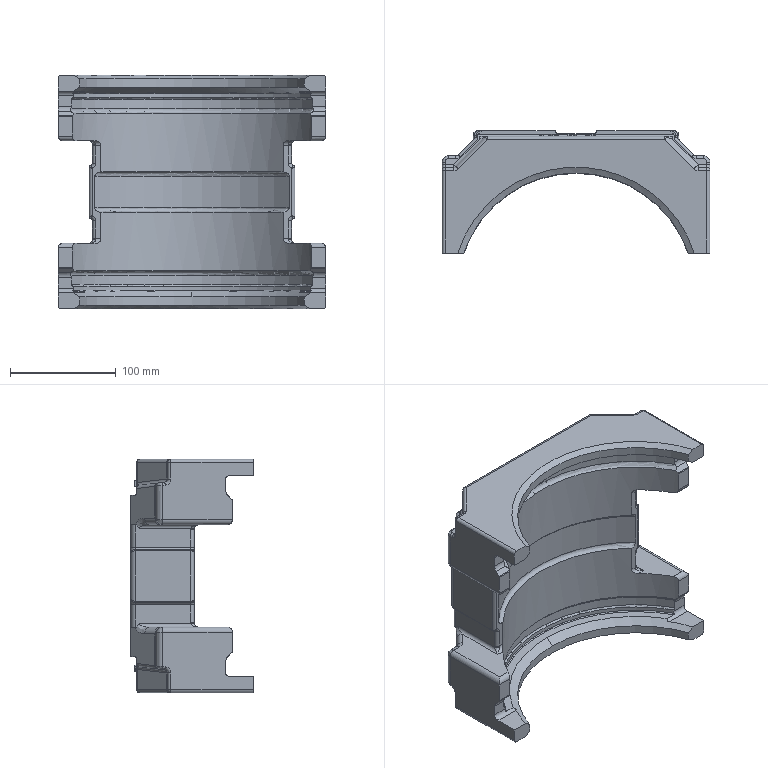Part | SolidWorks | features Fillet 8, Cut 5, Draft 4, MirrorPattern 3, Boss 2, RevCut 2, Extrusion 1 | 1 solid | 540 faces | box 253.206 x 115.888 x 220.663 mm | volume 2117949 mm3 | plane 274 | cylinder 129 | spline 87 | torus 32 | sphere 12 | cone 6 | commonest cylinder face diameters 6 x50 6.35 x14 3.175 x12 8.89 x12 12.7 x12 9.525 x10